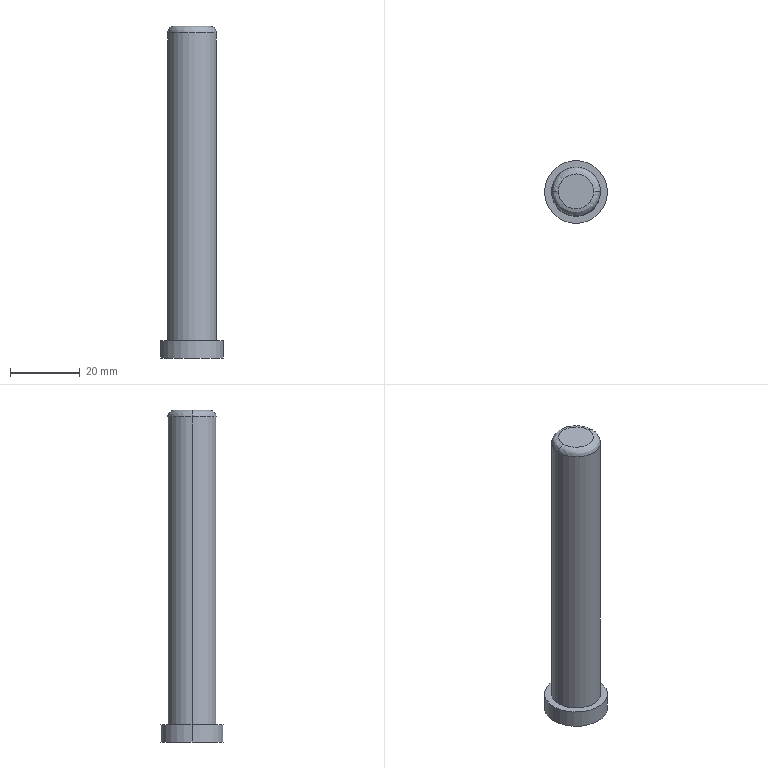Part | STEP file | CHOT DAN DUONG | 1 solid | 9 faces | box 18 x 18 x 95 mm | volume 15092 mm3 | cylinder 4 | plane 3 | spline 2 | commonest cylinder face diameters 14 x2 18 x2
STEP:
#1=CARTESIAN_POINT('',(0.,0.,0.));
#2=DIRECTION('',(0.,0.,1.));
#3=DIRECTION('',(1.,0.,0.));
#4=AXIS2_PLACEMENT_3D('',#1,#2,#3);
#5=CARTESIAN_POINT('',(7.,0.,93.));
#6=VERTEX_POINT('',#5);
#7=CARTESIAN_POINT('',(-7.,0.,93.));
#8=VERTEX_POINT('',#7);
#9=CARTESIAN_POINT('',(0.,0.,93.));
#10=DIRECTION('',(0.,0.,-1.));
#11=DIRECTION('',(1.,0.,0.));
#12=AXIS2_PLACEMENT_3D('',#9,#10,#11);
#13=CIRCLE('',#12,7.);
#14=CARTESIAN_POINT('',(7.,0.,93.));
#15=CARTESIAN_POINT('',(7.,-14.,93.));
#16=CARTESIAN_POINT('',(-7.,-14.,93.));
#17=CARTESIAN_POINT('',(-7.,0.,93.));
#18=CARTESIAN_POINT('',(7.,0.,94.172));
#19=CARTESIAN_POINT('',(7.,-14.,94.172));
#20=CARTESIAN_POINT('',(-7.,-14.,94.172));
#21=CARTESIAN_POINT('',(-7.,0.,94.172));
#22=CARTESIAN_POINT('',(6.172,0.,95.));
#23=CARTESIAN_POINT('',(6.172,-12.343,95.));
#24=CARTESIAN_POINT('',(-6.172,-12.343,95.));
#25=CARTESIAN_POINT('',(-6.172,0.,95.));
#26=CARTESIAN_POINT('',(5.,0.,95.));
#27=CARTESIAN_POINT('',(5.,-10.,95.));
#28=CARTESIAN_POINT('',(-5.,-10.,95.));
#29=CARTESIAN_POINT('',(-5.,0.,95.));
#30=(BOUNDED_SURFACE()B_SPLINE_SURFACE(3,3,((#14,#15,#16,#17),(#18,#19,#20,#21),(#22,#23,#24,#25),(#26,#27,#28,#29)),.UNSPECIFIED.,.F.,.F.,.F.)B_SPLINE_SURFACE_WITH_KNOTS((4,4),(4,4),(0.,1.),(0.,1.),.PIECEWISE_BEZIER_KNOTS.)GEOMETRIC_REPRESENTATION_ITEM()RATIONAL_B_SPLINE_SURFACE(((1.,0.3333,0.3333,1.),(0.8047,0.2682,0.2682,0.8047),(0.8047,0.2682,0.2682,0.8047),(1.,0.3333,0.3333,1.)))REPRESENTATION_ITEM('')SURFACE());
#31=CARTESIAN_POINT('',(0.,0.));
#32=CARTESIAN_POINT('',(0.,0.02375));
#33=CARTESIAN_POINT('',(0.,0.06805));
#34=CARTESIAN_POINT('',(0.,0.1267));
#35=CARTESIAN_POINT('',(0.,0.1794));
#36=CARTESIAN_POINT('',(0.,0.2276));
#37=CARTESIAN_POINT('',(0.,0.2721));
#38=CARTESIAN_POINT('',(0.,0.3139));
#39=CARTESIAN_POINT('',(0.,0.3535));
#40=CARTESIAN_POINT('',(0.,0.3914));
#41=CARTESIAN_POINT('',(0.,0.4282));
#42=CARTESIAN_POINT('',(0.,0.4643));
#43=CARTESIAN_POINT('',(0.,0.5));
#44=CARTESIAN_POINT('',(0.,0.5357));
#45=CARTESIAN_POINT('',(0.,0.5718));
#46=CARTESIAN_POINT('',(0.,0.6086));
#47=CARTESIAN_POINT('',(0.,0.6465));
#48=CARTESIAN_POINT('',(0.,0.6861));
#49=CARTESIAN_POINT('',(0.,0.7279));
#50=CARTESIAN_POINT('',(0.,0.7724));
#51=CARTESIAN_POINT('',(0.,0.8206));
#52=CARTESIAN_POINT('',(0.,0.8733));
#53=CARTESIAN_POINT('',(0.,0.9319));
#54=CARTESIAN_POINT('',(0.,0.9763));
#55=CARTESIAN_POINT('',(0.,1.));
#56=B_SPLINE_CURVE_WITH_KNOTS('',3,(#31,#32,#33,#34,#35,#36,#37,#38,#39,#40,#41,#42,#43,#44,#45,#46,#47,#48,#49,#50,#51,#52,#53,#54,#55),.UNSPECIFIED.,.F.,.F.,(4,1,1,1,1,1,1,1,1,1,1,1,1,1,1,1,1,1,1,1,1,1,4),(0.,0.1428,0.2856,0.4284,0.5712,0.714,0.8568,0.9996,1.142,1.285,1.428,1.571,1.714,1.856,1.999,2.142,2.285,2.428,2.57,2.713,2.856,2.999,3.142),.QUASI_UNIFORM_KNOTS.);
#57=(GEOMETRIC_REPRESENTATION_CONTEXT(2)PARAMETRIC_REPRESENTATION_CONTEXT()REPRESENTATION_CONTEXT('',''));
#58=DEFINITIONAL_REPRESENTATION('',(#56),#57);
#59=PCURVE('',#30,#58);
#60=CARTESIAN_POINT('',(0.,0.,5.));
#61=DIRECTION('',(0.,0.,1.));
#62=DIRECTION('',(1.,0.,0.));
#63=AXIS2_PLACEMENT_3D('',#60,#61,#62);
#64=CYLINDRICAL_SURFACE('',#63,7.);
#65=CARTESIAN_POINT('',(6.283,88.));
#66=DIRECTION('',(-1.,0.));
#67=VECTOR('',#66,1.);
#68=LINE('',#65,#67);
#69=(GEOMETRIC_REPRESENTATION_CONTEXT(2)PARAMETRIC_REPRESENTATION_CONTEXT()REPRESENTATION_CONTEXT('',''));
#70=DEFINITIONAL_REPRESENTATION('',(#68),#69);
#71=PCURVE('',#64,#70);
#72=SURFACE_CURVE('',#13,(#59,#71),.PCURVE_S1.);
#73=EDGE_CURVE('',#6,#8,#72,.T.);
#74=ORIENTED_EDGE('',*,*,#73,.F.);
#75=CARTESIAN_POINT('',(5.,0.,95.));
#76=VERTEX_POINT('',#75);
#77=CARTESIAN_POINT('',(5.,0.,93.));
#78=DIRECTION('',(0.,-1.,0.));
#79=DIRECTION('',(1.,0.,0.));
#80=AXIS2_PLACEMENT_3D('',#77,#78,#79);
#81=CIRCLE('',#80,2.);
#82=CARTESIAN_POINT('',(0.,0.));
#83=CARTESIAN_POINT('',(0.01683,0.));
#84=CARTESIAN_POINT('',(0.04999,0.));
#85=CARTESIAN_POINT('',(0.09843,0.));
#86=CARTESIAN_POINT('',(0.1457,0.));
#87=CARTESIAN_POINT('',(0.192,0.));
#88=CARTESIAN_POINT('',(0.2375,0.));
#89=CARTESIAN_POINT('',(0.2823,0.));
#90=CARTESIAN_POINT('',(0.3265,0.));
#91=CARTESIAN_POINT('',(0.3703,0.));
#92=CARTESIAN_POINT('',(0.4137,0.));
#93=CARTESIAN_POINT('',(0.4569,0.));
#94=CARTESIAN_POINT('',(0.5,0.));
#95=CARTESIAN_POINT('',(0.5431,0.));
#96=CARTESIAN_POINT('',(0.5863,0.));
#97=CARTESIAN_POINT('',(0.6297,0.));
#98=CARTESIAN_POINT('',(0.6735,0.));
#99=CARTESIAN_POINT('',(0.7177,0.));
#100=CARTESIAN_POINT('',(0.7625,0.));
#101=CARTESIAN_POINT('',(0.808,0.));
#102=CARTESIAN_POINT('',(0.8543,0.));
#103=CARTESIAN_POINT('',(0.9016,0.));
#104=CARTESIAN_POINT('',(0.95,0.));
#105=CARTESIAN_POINT('',(0.9832,0.));
#106=CARTESIAN_POINT('',(1.,0.));
#107=B_SPLINE_CURVE_WITH_KNOTS('',3,(#82,#83,#84,#85,#86,#87,#88,#89,#90,#91,#92,#93,#94,#95,#96,#97,#98,#99,#100,#101,#102,#103,#104,#105,#106),.UNSPECIFIED.,.F.,.F.,(4,1,1,1,1,1,1,1,1,1,1,1,1,1,1,1,1,1,1,1,1,1,4),(0.,0.0714,0.1428,0.2142,0.2856,0.357,0.4284,0.4998,0.5712,0.6426,0.714,0.7854,0.8568,0.9282,0.9996,1.071,1.142,1.214,1.285,1.357,1.428,1.499,1.571),.QUASI_UNIFORM_KNOTS.);
#108=(GEOMETRIC_REPRESENTATION_CONTEXT(2)PARAMETRIC_REPRESENTATION_CONTEXT()REPRESENTATION_CONTEXT('',''));
#109=DEFINITIONAL_REPRESENTATION('',(#107),#108);
#110=PCURVE('',#30,#109);
#111=CARTESIAN_POINT('',(-7.,0.,93.));
#112=CARTESIAN_POINT('',(-7.,14.,93.));
#113=CARTESIAN_POINT('',(7.,14.,93.));
#114=CARTESIAN_POINT('',(7.,0.,93.));
#115=CARTESIAN_POINT('',(-7.,0.,94.172));
#116=CARTESIAN_POINT('',(-7.,14.,94.172));
#117=CARTESIAN_POINT('',(7.,14.,94.172));
#118=CARTESIAN_POINT('',(7.,0.,94.172));
#119=CARTESIAN_POINT('',(-6.172,0.,95.));
#120=CARTESIAN_POINT('',(-6.172,12.343,95.));
#121=CARTESIAN_POINT('',(6.172,12.343,95.));
#122=CARTESIAN_POINT('',(6.172,0.,95.));
#123=CARTESIAN_POINT('',(-5.,0.,95.));
#124=CARTESIAN_POINT('',(-5.,10.,95.));
#125=CARTESIAN_POINT('',(5.,10.,95.));
#126=CARTESIAN_POINT('',(5.,0.,95.));
#127=(BOUNDED_SURFACE()B_SPLINE_SURFACE(3,3,((#111,#112,#113,#114),(#115,#116,#117,#118),(#119,#120,#121,#122),(#123,#124,#125,#126)),.UNSPECIFIED.,.F.,.F.,.F.)B_SPLINE_SURFACE_WITH_KNOTS((4,4),(4,4),(0.,1.),(0.,1.),.PIECEWISE_BEZIER_KNOTS.)GEOMETRIC_REPRESENTATION_ITEM()RATIONAL_B_SPLINE_SURFACE(((1.,0.3333,0.3333,1.),(0.8047,0.2682,0.2682,0.8047),(0.8047,0.2682,0.2682,0.8047),(1.,0.3333,0.3333,1.)))REPRESENTATION_ITEM('')SURFACE());
#128=CARTESIAN_POINT('',(0.,1.));
#129=CARTESIAN_POINT('',(0.01683,1.));
#130=CARTESIAN_POINT('',(0.04999,1.));
#131=CARTESIAN_POINT('',(0.09843,1.));
#132=CARTESIAN_POINT('',(0.1457,1.));
#133=CARTESIAN_POINT('',(0.192,1.));
#134=CARTESIAN_POINT('',(0.2375,1.));
#135=CARTESIAN_POINT('',(0.2823,1.));
#136=CARTESIAN_POINT('',(0.3265,1.));
#137=CARTESIAN_POINT('',(0.3703,1.));
#138=CARTESIAN_POINT('',(0.4137,1.));
#139=CARTESIAN_POINT('',(0.4569,1.));
#140=CARTESIAN_POINT('',(0.5,1.));
#141=CARTESIAN_POINT('',(0.5431,1.));
#142=CARTESIAN_POINT('',(0.5863,1.));
#143=CARTESIAN_POINT('',(0.6297,1.));
#144=CARTESIAN_POINT('',(0.6735,1.));
#145=CARTESIAN_POINT('',(0.7177,1.));
#146=CARTESIAN_POINT('',(0.7625,1.));
#147=CARTESIAN_POINT('',(0.808,1.));
#148=CARTESIAN_POINT('',(0.8543,1.));
#149=CARTESIAN_POINT('',(0.9016,1.));
#150=CARTESIAN_POINT('',(0.95,1.));
#151=CARTESIAN_POINT('',(0.9832,1.));
#152=CARTESIAN_POINT('',(1.,1.));
#153=B_SPLINE_CURVE_WITH_KNOTS('',3,(#128,#129,#130,#131,#132,#133,#134,#135,#136,#137,#138,#139,#140,#141,#142,#143,#144,#145,#146,#147,#148,#149,#150,#151,#152),.UNSPECIFIED.,.F.,.F.,(4,1,1,1,1,1,1,1,1,1,1,1,1,1,1,1,1,1,1,1,1,1,4),(0.,0.0714,0.1428,0.2142,0.2856,0.357,0.4284,0.4998,0.5712,0.6426,0.714,0.7854,0.8568,0.9282,0.9996,1.071,1.142,1.214,1.285,1.357,1.428,1.499,1.571),.QUASI_UNIFORM_KNOTS.);
#154=(GEOMETRIC_REPRESENTATION_CONTEXT(2)PARAMETRIC_REPRESENTATION_CONTEXT()REPRESENTATION_CONTEXT('',''));
#155=DEFINITIONAL_REPRESENTATION('',(#153),#154);
#156=PCURVE('',#127,#155);
#157=SURFACE_CURVE('',#81,(#110,#156),.PCURVE_S1.);
#158=EDGE_CURVE('',#6,#76,#157,.T.);
#159=ORIENTED_EDGE('',*,*,#158,.T.);
#160=CARTESIAN_POINT('',(-5.,0.,95.));
#161=VERTEX_POINT('',#160);
#162=CARTESIAN_POINT('',(5.,0.,95.));
#163=CARTESIAN_POINT('',(5.,-10.,95.));
#164=CARTESIAN_POINT('',(-5.,-10.,95.));
#165=CARTESIAN_POINT('',(-5.,0.,95.));
#166=(BOUNDED_CURVE()B_SPLINE_CURVE(3,(#162,#163,#164,#165),.UNSPECIFIED.,.F.,.F.)B_SPLINE_CURVE_WITH_KNOTS((4,4),(0.,0.5),.PIECEWISE_BEZIER_KNOTS.)CURVE()GEOMETRIC_REPRESENTATION_ITEM()RATIONAL_B_SPLINE_CURVE((1.,0.3333,0.3333,1.))REPRESENTATION_ITEM(''));
#167=CARTESIAN_POINT('',(1.,0.));
#168=CARTESIAN_POINT('',(1.,1.));
#169=B_SPLINE_CURVE_WITH_KNOTS('',1,(#167,#168),.UNSPECIFIED.,.F.,.F.,(2,2),(0.,0.5),.PIECEWISE_BEZIER_KNOTS.);
#170=(GEOMETRIC_REPRESENTATION_CONTEXT(2)PARAMETRIC_REPRESENTATION_CONTEXT()REPRESENTATION_CONTEXT('',''));
#171=DEFINITIONAL_REPRESENTATION('',(#169),#170);
#172=PCURVE('',#30,#171);
#173=CARTESIAN_POINT('',(0.,0.,95.));
#174=DIRECTION('',(0.,0.,-1.));
#175=DIRECTION('',(-1.,0.,0.));
#176=AXIS2_PLACEMENT_3D('',#173,#174,#175);
#177=PLANE('',#176);
#178=CARTESIAN_POINT('',(-5.,0.));
#179=CARTESIAN_POINT('',(-5.,-10.));
#180=CARTESIAN_POINT('',(5.,-10.));
#181=CARTESIAN_POINT('',(5.,0.));
#182=(BOUNDED_CURVE()B_SPLINE_CURVE(3,(#178,#179,#180,#181),.UNSPECIFIED.,.F.,.F.)B_SPLINE_CURVE_WITH_KNOTS((4,4),(0.,0.5),.PIECEWISE_BEZIER_KNOTS.)CURVE()GEOMETRIC_REPRESENTATION_ITEM()RATIONAL_B_SPLINE_CURVE((1.,0.3333,0.3333,1.))REPRESENTATION_ITEM(''));
#183=(GEOMETRIC_REPRESENTATION_CONTEXT(2)PARAMETRIC_REPRESENTATION_CONTEXT()REPRESENTATION_CONTEXT('',''));
#184=DEFINITIONAL_REPRESENTATION('',(#182),#183);
#185=PCURVE('',#177,#184);
#186=SURFACE_CURVE('',#166,(#172,#185),.PCURVE_S1.);
#187=EDGE_CURVE('',#76,#161,#186,.T.);
#188=ORIENTED_EDGE('',*,*,#187,.T.);
#189=CARTESIAN_POINT('',(-5.,0.,93.));
#190=DIRECTION('',(0.,1.,0.));
#191=DIRECTION('',(-1.,0.,0.));
#192=AXIS2_PLACEMENT_3D('',#189,#190,#191);
#193=CIRCLE('',#192,2.);
#194=CARTESIAN_POINT('',(0.,1.));
#195=CARTESIAN_POINT('',(0.01683,1.));
#196=CARTESIAN_POINT('',(0.04999,1.));
#197=CARTESIAN_POINT('',(0.09843,1.));
#198=CARTESIAN_POINT('',(0.1457,1.));
#199=CARTESIAN_POINT('',(0.192,1.));
#200=CARTESIAN_POINT('',(0.2375,1.));
#201=CARTESIAN_POINT('',(0.2823,1.));
#202=CARTESIAN_POINT('',(0.3265,1.));
#203=CARTESIAN_POINT('',(0.3703,1.));
#204=CARTESIAN_POINT('',(0.4137,1.));
#205=CARTESIAN_POINT('',(0.4569,1.));
#206=CARTESIAN_POINT('',(0.5,1.));
#207=CARTESIAN_POINT('',(0.5431,1.));
#208=CARTESIAN_POINT('',(0.5863,1.));
#209=CARTESIAN_POINT('',(0.6297,1.));
#210=CARTESIAN_POINT('',(0.6735,1.));
#211=CARTESIAN_POINT('',(0.7177,1.));
#212=CARTESIAN_POINT('',(0.7625,1.));
#213=CARTESIAN_POINT('',(0.808,1.));
#214=CARTESIAN_POINT('',(0.8543,1.));
#215=CARTESIAN_POINT('',(0.9016,1.));
#216=CARTESIAN_POINT('',(0.95,1.));
#217=CARTESIAN_POINT('',(0.9832,1.));
#218=CARTESIAN_POINT('',(1.,1.));
#219=B_SPLINE_CURVE_WITH_KNOTS('',3,(#194,#195,#196,#197,#198,#199,#200,#201,#202,#203,#204,#205,#206,#207,#208,#209,#210,#211,#212,#213,#214,#215,#216,#217,#218),.UNSPECIFIED.,.F.,.F.,(4,1,1,1,1,1,1,1,1,1,1,1,1,1,1,1,1,1,1,1,1,1,4),(0.,0.0714,0.1428,0.2142,0.2856,0.357,0.4284,0.4998,0.5712,0.6426,0.714,0.7854,0.8568,0.9282,0.9996,1.071,1.142,1.214,1.285,1.357,1.428,1.499,1.571),.QUASI_UNIFORM_KNOTS.);
#220=(GEOMETRIC_REPRESENTATION_CONTEXT(2)PARAMETRIC_REPRESENTATION_CONTEXT()REPRESENTATION_CONTEXT('',''));
#221=DEFINITIONAL_REPRESENTATION('',(#219),#220);
#222=PCURVE('',#30,#221);
#223=CARTESIAN_POINT('',(0.,0.));
#224=CARTESIAN_POINT('',(0.01683,0.));
#225=CARTESIAN_POINT('',(0.04999,0.));
#226=CARTESIAN_POINT('',(0.09843,0.));
#227=CARTESIAN_POINT('',(0.1457,0.));
#228=CARTESIAN_POINT('',(0.192,0.));
#229=CARTESIAN_POINT('',(0.2375,0.));
#230=CARTESIAN_POINT('',(0.2823,0.));
#231=CARTESIAN_POINT('',(0.3265,0.));
#232=CARTESIAN_POINT('',(0.3703,0.));
#233=CARTESIAN_POINT('',(0.4137,0.));
#234=CARTESIAN_POINT('',(0.4569,0.));
#235=CARTESIAN_POINT('',(0.5,0.));
#236=CARTESIAN_POINT('',(0.5431,0.));
#237=CARTESIAN_POINT('',(0.5863,0.));
#238=CARTESIAN_POINT('',(0.6297,0.));
#239=CARTESIAN_POINT('',(0.6735,0.));
#240=CARTESIAN_POINT('',(0.7177,0.));
#241=CARTESIAN_POINT('',(0.7625,0.));
#242=CARTESIAN_POINT('',(0.808,0.));
#243=CARTESIAN_POINT('',(0.8543,0.));
#244=CARTESIAN_POINT('',(0.9016,0.));
#245=CARTESIAN_POINT('',(0.95,0.));
#246=CARTESIAN_POINT('',(0.9832,0.));
#247=CARTESIAN_POINT('',(1.,0.));
#248=B_SPLINE_CURVE_WITH_KNOTS('',3,(#223,#224,#225,#226,#227,#228,#229,#230,#231,#232,#233,#234,#235,#236,#237,#238,#239,#240,#241,#242,#243,#244,#245,#246,#247),.UNSPECIFIED.,.F.,.F.,(4,1,1,1,1,1,1,1,1,1,1,1,1,1,1,1,1,1,1,1,1,1,4),(0.,0.0714,0.1428,0.2142,0.2856,0.357,0.4284,0.4998,0.5712,0.6426,0.714,0.7854,0.8568,0.9282,0.9996,1.071,1.142,1.214,1.285,1.357,1.428,1.499,1.571),.QUASI_UNIFORM_KNOTS.);
#249=(GEOMETRIC_REPRESENTATION_CONTEXT(2)PARAMETRIC_REPRESENTATION_CONTEXT()REPRESENTATION_CONTEXT('',''));
#250=DEFINITIONAL_REPRESENTATION('',(#248),#249);
#251=PCURVE('',#127,#250);
#252=SURFACE_CURVE('',#193,(#222,#251),.PCURVE_S1.);
#253=EDGE_CURVE('',#8,#161,#252,.T.);
#254=ORIENTED_EDGE('',*,*,#253,.F.);
#255=EDGE_LOOP('',(#74,#159,#188,#254));
#256=FACE_BOUND('',#255,.T.);
#257=ADVANCED_FACE('',(#256),#30,.T.);
#258=CARTESIAN_POINT('',(7.,0.,5.));
#259=VERTEX_POINT('',#258);
#260=CARTESIAN_POINT('',(-7.,0.,5.));
#261=VERTEX_POINT('',#260);
#262=CARTESIAN_POINT('',(0.,0.,5.));
#263=DIRECTION('',(0.,0.,1.));
#264=DIRECTION('',(1.,0.,0.));
#265=AXIS2_PLACEMENT_3D('',#262,#263,#264);
#266=CIRCLE('',#265,7.);
#267=CARTESIAN_POINT('',(0.,0.,5.));
#268=DIRECTION('',(0.,0.,1.));
#269=DIRECTION('',(1.,0.,0.));
#270=AXIS2_PLACEMENT_3D('',#267,#268,#269);
#271=CYLINDRICAL_SURFACE('',#270,7.);
#272=CARTESIAN_POINT('',(0.,0.));
#273=DIRECTION('',(1.,0.));
#274=VECTOR('',#273,1.);
#275=LINE('',#272,#274);
#276=(GEOMETRIC_REPRESENTATION_CONTEXT(2)PARAMETRIC_REPRESENTATION_CONTEXT()REPRESENTATION_CONTEXT('',''));
#277=DEFINITIONAL_REPRESENTATION('',(#275),#276);
#278=PCURVE('',#271,#277);
#279=CARTESIAN_POINT('',(0.,0.,5.));
#280=DIRECTION('',(0.,0.,-1.));
#281=DIRECTION('',(-1.,0.,0.));
#282=AXIS2_PLACEMENT_3D('',#279,#280,#281);
#283=PLANE('',#282);
#284=CARTESIAN_POINT('',(-7.,0.));
#285=CARTESIAN_POINT('',(-7.,12.124));
#286=CARTESIAN_POINT('',(3.5,6.062));
#287=CARTESIAN_POINT('',(14.,0.));
#288=CARTESIAN_POINT('',(3.5,-6.062));
#289=CARTESIAN_POINT('',(-7.,-12.124));
#290=CARTESIAN_POINT('',(-7.,0.));
#291=(BOUNDED_CURVE()B_SPLINE_CURVE(2,(#284,#285,#286,#287,#288,#289,#290),.UNSPECIFIED.,.T.,.F.)B_SPLINE_CURVE_WITH_KNOTS((1,2,2,2,2,1),(-2.094,0.,2.094,4.189,6.283,8.378),.UNSPECIFIED.)CURVE()GEOMETRIC_REPRESENTATION_ITEM()RATIONAL_B_SPLINE_CURVE((1.,0.5,1.,0.5,1.,0.5,1.))REPRESENTATION_ITEM(''));
#292=(GEOMETRIC_REPRESENTATION_CONTEXT(2)PARAMETRIC_REPRESENTATION_CONTEXT()REPRESENTATION_CONTEXT('',''));
#293=DEFINITIONAL_REPRESENTATION('',(#291),#292);
#294=PCURVE('',#283,#293);
#295=SURFACE_CURVE('',#266,(#278,#294),.PCURVE_S1.);
#296=EDGE_CURVE('',#259,#261,#295,.T.);
#297=ORIENTED_EDGE('',*,*,#296,.T.);
#298=CARTESIAN_POINT('',(-7.,0.,5.));
#299=DIRECTION('',(0.,0.,1.));
#300=VECTOR('',#299,1.);
#301=LINE('',#298,#300);
#302=CARTESIAN_POINT('',(3.142,0.));
#303=DIRECTION('',(0.,1.));
#304=VECTOR('',#303,1.);
#305=LINE('',#302,#304);
#306=(GEOMETRIC_REPRESENTATION_CONTEXT(2)PARAMETRIC_REPRESENTATION_CONTEXT()REPRESENTATION_CONTEXT('',''));
#307=DEFINITIONAL_REPRESENTATION('',(#305),#306);
#308=PCURVE('',#271,#307);
#309=CARTESIAN_POINT('',(3.142,0.));
#310=DIRECTION('',(0.,1.));
#311=VECTOR('',#310,1.);
#312=LINE('',#309,#311);
#313=(GEOMETRIC_REPRESENTATION_CONTEXT(2)PARAMETRIC_REPRESENTATION_CONTEXT()REPRESENTATION_CONTEXT('',''));
#314=DEFINITIONAL_REPRESENTATION('',(#312),#313);
#315=PCURVE('',#64,#314);
#316=SURFACE_CURVE('',#301,(#308,#315),.PCURVE_S1.);
#317=EDGE_CURVE('',#261,#8,#316,.T.);
#318=ORIENTED_EDGE('',*,*,#317,.T.);
#319=CARTESIAN_POINT('',(0.,0.,93.));
#320=DIRECTION('',(0.,0.,-1.));
#321=DIRECTION('',(1.,0.,0.));
#322=AXIS2_PLACEMENT_3D('',#319,#320,#321);
#323=CIRCLE('',#322,7.);
#324=CARTESIAN_POINT('',(6.283,88.));
#325=DIRECTION('',(-1.,0.));
#326=VECTOR('',#325,1.);
#327=LINE('',#324,#326);
#328=(GEOMETRIC_REPRESENTATION_CONTEXT(2)PARAMETRIC_REPRESENTATION_CONTEXT()REPRESENTATION_CONTEXT('',''));
#329=DEFINITIONAL_REPRESENTATION('',(#327),#328);
#330=PCURVE('',#271,#329);
#331=CARTESIAN_POINT('',(0.,0.));
#332=CARTESIAN_POINT('',(0.,0.02375));
#333=CARTESIAN_POINT('',(0.,0.06805));
#334=CARTESIAN_POINT('',(0.,0.1267));
#335=CARTESIAN_POINT('',(0.,0.1794));
#336=CARTESIAN_POINT('',(0.,0.2276));
#337=CARTESIAN_POINT('',(0.,0.2721));
#338=CARTESIAN_POINT('',(0.,0.3139));
#339=CARTESIAN_POINT('',(0.,0.3535));
#340=CARTESIAN_POINT('',(0.,0.3914));
#341=CARTESIAN_POINT('',(0.,0.4282));
#342=CARTESIAN_POINT('',(0.,0.4643));
#343=CARTESIAN_POINT('',(0.,0.5));
#344=CARTESIAN_POINT('',(0.,0.5357));
#345=CARTESIAN_POINT('',(0.,0.5718));
#346=CARTESIAN_POINT('',(0.,0.6086));
#347=CARTESIAN_POINT('',(0.,0.6465));
#348=CARTESIAN_POINT('',(0.,0.6861));
#349=CARTESIAN_POINT('',(0.,0.7279));
#350=CARTESIAN_POINT('',(0.,0.7724));
#351=CARTESIAN_POINT('',(0.,0.8206));
#352=CARTESIAN_POINT('',(0.,0.8733));
#353=CARTESIAN_POINT('',(0.,0.9319));
#354=CARTESIAN_POINT('',(0.,0.9763));
#355=CARTESIAN_POINT('',(0.,1.));
#356=B_SPLINE_CURVE_WITH_KNOTS('',3,(#331,#332,#333,#334,#335,#336,#337,#338,#339,#340,#341,#342,#343,#344,#345,#346,#347,#348,#349,#350,#351,#352,#353,#354,#355),.UNSPECIFIED.,.F.,.F.,(4,1,1,1,1,1,1,1,1,1,1,1,1,1,1,1,1,1,1,1,1,1,4),(3.142,3.284,3.427,3.57,3.713,3.856,3.998,4.141,4.284,4.427,4.57,4.712,4.855,4.998,5.141,5.284,5.426,5.569,5.712,5.855,5.998,6.14,6.283),.QUASI_UNIFORM_KNOTS.);
#357=(GEOMETRIC_REPRESENTATION_CONTEXT(2)PARAMETRIC_REPRESENTATION_CONTEXT()REPRESENTATION_CONTEXT('',''));
#358=DEFINITIONAL_REPRESENTATION('',(#356),#357);
#359=PCURVE('',#127,#358);
#360=SURFACE_CURVE('',#323,(#330,#359),.PCURVE_S1.);
#361=EDGE_CURVE('',#8,#6,#360,.T.);
#362=ORIENTED_EDGE('',*,*,#361,.T.);
#363=CARTESIAN_POINT('',(7.,0.,5.));
#364=DIRECTION('',(0.,0.,1.));
#365=VECTOR('',#364,1.);
#366=LINE('',#363,#365);
#367=CARTESIAN_POINT('',(0.,0.));
#368=DIRECTION('',(0.,1.));
#369=VECTOR('',#368,1.);
#370=LINE('',#367,#369);
#371=(GEOMETRIC_REPRESENTATION_CONTEXT(2)PARAMETRIC_REPRESENTATION_CONTEXT()REPRESENTATION_CONTEXT('',''));
#372=DEFINITIONAL_REPRESENTATION('',(#370),#371);
#373=PCURVE('',#271,#372);
#374=CARTESIAN_POINT('',(6.283,0.));
#375=DIRECTION('',(0.,1.));
#376=VECTOR('',#375,1.);
#377=LINE('',#374,#376);
#378=(GEOMETRIC_REPRESENTATION_CONTEXT(2)PARAMETRIC_REPRESENTATION_CONTEXT()REPRESENTATION_CONTEXT('',''));
#379=DEFINITIONAL_REPRESENTATION('',(#377),#378);
#380=PCURVE('',#64,#379);
#381=SURFACE_CURVE('',#366,(#373,#380),.PCURVE_S1.);
#382=EDGE_CURVE('',#259,#6,#381,.T.);
#383=ORIENTED_EDGE('',*,*,#382,.F.);
#384=EDGE_LOOP('',(#297,#318,#362,#383));
#385=FACE_BOUND('',#384,.T.);
#386=ADVANCED_FACE('',(#385),#271,.T.);
#387=CARTESIAN_POINT('',(9.,0.,0.));
#388=VERTEX_POINT('',#387);
#389=CARTESIAN_POINT('',(-9.,0.,0.));
#390=VERTEX_POINT('',#389);
#391=CARTESIAN_POINT('',(0.,0.,0.));
#392=DIRECTION('',(0.,0.,1.));
#393=DIRECTION('',(1.,0.,0.));
#394=AXIS2_PLACEMENT_3D('',#391,#392,#393);
#395=CIRCLE('',#394,9.);
#396=CARTESIAN_POINT('',(0.,0.,0.));
#397=DIRECTION('',(0.,0.,1.));
#398=DIRECTION('',(1.,0.,0.));
#399=AXIS2_PLACEMENT_3D('',#396,#397,#398);
#400=CYLINDRICAL_SURFACE('',#399,9.);
#401=CARTESIAN_POINT('',(0.,0.));
#402=DIRECTION('',(1.,0.));
#403=VECTOR('',#402,1.);
#404=LINE('',#401,#403);
#405=(GEOMETRIC_REPRESENTATION_CONTEXT(2)PARAMETRIC_REPRESENTATION_CONTEXT()REPRESENTATION_CONTEXT('',''));
#406=DEFINITIONAL_REPRESENTATION('',(#404),#405);
#407=PCURVE('',#400,#406);
#408=CARTESIAN_POINT('',(0.,0.,0.));
#409=DIRECTION('',(0.,0.,-1.));
#410=DIRECTION('',(-1.,0.,0.));
#411=AXIS2_PLACEMENT_3D('',#408,#409,#410);
#412=PLANE('',#411);
#413=CARTESIAN_POINT('',(-9.,0.));
#414=CARTESIAN_POINT('',(-9.,15.588));
#415=CARTESIAN_POINT('',(4.5,7.794));
#416=CARTESIAN_POINT('',(18.,0.));
#417=CARTESIAN_POINT('',(4.5,-7.794));
#418=CARTESIAN_POINT('',(-9.,-15.588));
#419=CARTESIAN_POINT('',(-9.,0.));
#420=(BOUNDED_CURVE()B_SPLINE_CURVE(2,(#413,#414,#415,#416,#417,#418,#419),.UNSPECIFIED.,.T.,.F.)B_SPLINE_CURVE_WITH_KNOTS((1,2,2,2,2,1),(-2.094,0.,2.094,4.189,6.283,8.378),.UNSPECIFIED.)CURVE()GEOMETRIC_REPRESENTATION_ITEM()RATIONAL_B_SPLINE_CURVE((1.,0.5,1.,0.5,1.,0.5,1.))REPRESENTATION_ITEM(''));
#421=(GEOMETRIC_REPRESENTATION_CONTEXT(2)PARAMETRIC_REPRESENTATION_CONTEXT()REPRESENTATION_CONTEXT('',''));
#422=DEFINITIONAL_REPRESENTATION('',(#420),#421);
#423=PCURVE('',#412,#422);
#424=SURFACE_CURVE('',#395,(#407,#423),.PCURVE_S1.);
#425=EDGE_CURVE('',#388,#390,#424,.T.);
#426=ORIENTED_EDGE('',*,*,#425,.T.);
#427=CARTESIAN_POINT('',(-9.,0.,5.));
#428=VERTEX_POINT('',#427);
#429=CARTESIAN_POINT('',(-9.,0.,0.));
#430=DIRECTION('',(0.,0.,1.));
#431=VECTOR('',#430,1.);
#432=LINE('',#429,#431);
#433=CARTESIAN_POINT('',(3.142,0.));
#434=DIRECTION('',(0.,1.));
#435=VECTOR('',#434,1.);
#436=LINE('',#433,#435);
#437=(GEOMETRIC_REPRESENTATION_CONTEXT(2)PARAMETRIC_REPRESENTATION_CONTEXT()REPRESENTATION_CONTEXT('',''));
#438=DEFINITIONAL_REPRESENTATION('',(#436),#437);
#439=PCURVE('',#400,#438);
#440=CARTESIAN_POINT('',(0.,0.,0.));
#441=DIRECTION('',(0.,0.,1.));
#442=DIRECTION('',(1.,0.,0.));
#443=AXIS2_PLACEMENT_3D('',#440,#441,#442);
#444=CYLINDRICAL_SURFACE('',#443,9.);
#445=CARTESIAN_POINT('',(3.142,0.));
#446=DIRECTION('',(0.,1.));
#447=VECTOR('',#446,1.);
#448=LINE('',#445,#447);
#449=(GEOMETRIC_REPRESENTATION_CONTEXT(2)PARAMETRIC_REPRESENTATION_CONTEXT()REPRESENTATION_CONTEXT('',''));
#450=DEFINITIONAL_REPRESENTATION('',(#448),#449);
#451=PCURVE('',#444,#450);
#452=SURFACE_CURVE('',#432,(#439,#451),.PCURVE_S1.);
#453=EDGE_CURVE('',#390,#428,#452,.T.);
#454=ORIENTED_EDGE('',*,*,#453,.T.);
#455=CARTESIAN_POINT('',(9.,0.,5.));
#456=VERTEX_POINT('',#455);
#457=CARTESIAN_POINT('',(0.,0.,5.));
#458=DIRECTION('',(0.,0.,-1.));
#459=DIRECTION('',(1.,0.,0.));
#460=AXIS2_PLACEMENT_3D('',#457,#458,#459);
#461=CIRCLE('',#460,9.);
#462=CARTESIAN_POINT('',(6.283,5.));
#463=DIRECTION('',(-1.,0.));
#464=VECTOR('',#463,1.);
#465=LINE('',#462,#464);
#466=(GEOMETRIC_REPRESENTATION_CONTEXT(2)PARAMETRIC_REPRESENTATION_CONTEXT()REPRESENTATION_CONTEXT('',''));
#467=DEFINITIONAL_REPRESENTATION('',(#465),#466);
#468=PCURVE('',#400,#467);
#469=CARTESIAN_POINT('',(0.,0.));
#470=DIRECTION('',(-1.,0.));
#471=AXIS2_PLACEMENT_2D('',#469,#470);
#472=CIRCLE('',#471,9.);
#473=(GEOMETRIC_REPRESENTATION_CONTEXT(2)PARAMETRIC_REPRESENTATION_CONTEXT()REPRESENTATION_CONTEXT('',''));
#474=DEFINITIONAL_REPRESENTATION('',(#472),#473);
#475=PCURVE('',#283,#474);
#476=SURFACE_CURVE('',#461,(#468,#475),.PCURVE_S1.);
#477=EDGE_CURVE('',#428,#456,#476,.T.);
#478=ORIENTED_EDGE('',*,*,#477,.T.);
#479=CARTESIAN_POINT('',(9.,0.,0.));
#480=DIRECTION('',(0.,0.,1.));
#481=VECTOR('',#480,1.);
#482=LINE('',#479,#481);
#483=CARTESIAN_POINT('',(0.,0.));
#484=DIRECTION('',(0.,1.));
#485=VECTOR('',#484,1.);
#486=LINE('',#483,#485);
#487=(GEOMETRIC_REPRESENTATION_CONTEXT(2)PARAMETRIC_REPRESENTATION_CONTEXT()REPRESENTATION_CONTEXT('',''));
#488=DEFINITIONAL_REPRESENTATION('',(#486),#487);
#489=PCURVE('',#400,#488);
#490=CARTESIAN_POINT('',(6.283,0.));
#491=DIRECTION('',(0.,1.));
#492=VECTOR('',#491,1.);
#493=LINE('',#490,#492);
#494=(GEOMETRIC_REPRESENTATION_CONTEXT(2)PARAMETRIC_REPRESENTATION_CONTEXT()REPRESENTATION_CONTEXT('',''));
#495=DEFINITIONAL_REPRESENTATION('',(#493),#494);
#496=PCURVE('',#444,#495);
#497=SURFACE_CURVE('',#482,(#489,#496),.PCURVE_S1.);
#498=EDGE_CURVE('',#388,#456,#497,.T.);
#499=ORIENTED_EDGE('',*,*,#498,.F.);
#500=EDGE_LOOP('',(#426,#454,#478,#499));
#501=FACE_BOUND('',#500,.T.);
#502=ADVANCED_FACE('',(#501),#400,.T.);
#503=ORIENTED_EDGE('',*,*,#317,.F.);
#504=CARTESIAN_POINT('',(0.,0.,5.));
#505=DIRECTION('',(0.,0.,1.));
#506=DIRECTION('',(1.,0.,0.));
#507=AXIS2_PLACEMENT_3D('',#504,#505,#506);
#508=CIRCLE('',#507,7.);
#509=CARTESIAN_POINT('',(0.,0.));
#510=DIRECTION('',(1.,0.));
#511=VECTOR('',#510,1.);
#512=LINE('',#509,#511);
#513=(GEOMETRIC_REPRESENTATION_CONTEXT(2)PARAMETRIC_REPRESENTATION_CONTEXT()REPRESENTATION_CONTEXT('',''));
#514=DEFINITIONAL_REPRESENTATION('',(#512),#513);
#515=PCURVE('',#64,#514);
#516=CARTESIAN_POINT('',(-7.,0.));
#517=CARTESIAN_POINT('',(-7.,12.124));
#518=CARTESIAN_POINT('',(3.5,6.062));
#519=CARTESIAN_POINT('',(14.,0.));
#520=CARTESIAN_POINT('',(3.5,-6.062));
#521=CARTESIAN_POINT('',(-7.,-12.124));
#522=CARTESIAN_POINT('',(-7.,0.));
#523=(BOUNDED_CURVE()B_SPLINE_CURVE(2,(#516,#517,#518,#519,#520,#521,#522),.UNSPECIFIED.,.T.,.F.)B_SPLINE_CURVE_WITH_KNOTS((1,2,2,2,2,1),(-2.094,0.,2.094,4.189,6.283,8.378),.UNSPECIFIED.)CURVE()GEOMETRIC_REPRESENTATION_ITEM()RATIONAL_B_SPLINE_CURVE((1.,0.5,1.,0.5,1.,0.5,1.))REPRESENTATION_ITEM(''));
#524=(GEOMETRIC_REPRESENTATION_CONTEXT(2)PARAMETRIC_REPRESENTATION_CONTEXT()REPRESENTATION_CONTEXT('',''));
#525=DEFINITIONAL_REPRESENTATION('',(#523),#524);
#526=PCURVE('',#283,#525);
#527=SURFACE_CURVE('',#508,(#515,#526),.PCURVE_S1.);
#528=EDGE_CURVE('',#261,#259,#527,.T.);
#529=ORIENTED_EDGE('',*,*,#528,.T.);
#530=ORIENTED_EDGE('',*,*,#382,.T.);
#531=ORIENTED_EDGE('',*,*,#73,.T.);
#532=EDGE_LOOP('',(#503,#529,#530,#531));
#533=FACE_BOUND('',#532,.T.);
#534=ADVANCED_FACE('',(#533),#64,.T.);
#535=ORIENTED_EDGE('',*,*,#158,.F.);
#536=ORIENTED_EDGE('',*,*,#361,.F.);
#537=ORIENTED_EDGE('',*,*,#253,.T.);
#538=CARTESIAN_POINT('',(-5.,0.,95.));
#539=CARTESIAN_POINT('',(-5.,10.,95.));
#540=CARTESIAN_POINT('',(5.,10.,95.));
#541=CARTESIAN_POINT('',(5.,0.,95.));
#542=(BOUNDED_CURVE()B_SPLINE_CURVE(3,(#538,#539,#540,#541),.UNSPECIFIED.,.F.,.F.)B_SPLINE_CURVE_WITH_KNOTS((4,4),(0.5,1.),.PIECEWISE_BEZIER_KNOTS.)CURVE()GEOMETRIC_REPRESENTATION_ITEM()RATIONAL_B_SPLINE_CURVE((1.,0.3333,0.3333,1.))REPRESENTATION_ITEM(''));
#543=CARTESIAN_POINT('',(1.,0.));
#544=CARTESIAN_POINT('',(1.,1.));
#545=B_SPLINE_CURVE_WITH_KNOTS('',1,(#543,#544),.UNSPECIFIED.,.F.,.F.,(2,2),(0.5,1.),.PIECEWISE_BEZIER_KNOTS.);
#546=(GEOMETRIC_REPRESENTATION_CONTEXT(2)PARAMETRIC_REPRESENTATION_CONTEXT()REPRESENTATION_CONTEXT('',''));
#547=DEFINITIONAL_REPRESENTATION('',(#545),#546);
#548=PCURVE('',#127,#547);
#549=CARTESIAN_POINT('',(5.,0.));
#550=CARTESIAN_POINT('',(5.,10.));
#551=CARTESIAN_POINT('',(-5.,10.));
#552=CARTESIAN_POINT('',(-5.,0.));
#553=(BOUNDED_CURVE()B_SPLINE_CURVE(3,(#549,#550,#551,#552),.UNSPECIFIED.,.F.,.F.)B_SPLINE_CURVE_WITH_KNOTS((4,4),(0.5,1.),.PIECEWISE_BEZIER_KNOTS.)CURVE()GEOMETRIC_REPRESENTATION_ITEM()RATIONAL_B_SPLINE_CURVE((1.,0.3333,0.3333,1.))REPRESENTATION_ITEM(''));
#554=(GEOMETRIC_REPRESENTATION_CONTEXT(2)PARAMETRIC_REPRESENTATION_CONTEXT()REPRESENTATION_CONTEXT('',''));
#555=DEFINITIONAL_REPRESENTATION('',(#553),#554);
#556=PCURVE('',#177,#555);
#557=SURFACE_CURVE('',#542,(#548,#556),.PCURVE_S1.);
#558=EDGE_CURVE('',#161,#76,#557,.T.);
#559=ORIENTED_EDGE('',*,*,#558,.T.);
#560=EDGE_LOOP('',(#535,#536,#537,#559));
#561=FACE_BOUND('',#560,.T.);
#562=ADVANCED_FACE('',(#561),#127,.T.);
#563=ORIENTED_EDGE('',*,*,#296,.F.);
#564=ORIENTED_EDGE('',*,*,#528,.F.);
#565=EDGE_LOOP('',(#563,#564));
#566=FACE_BOUND('',#565,.T.);
#567=CARTESIAN_POINT('',(0.,0.,5.));
#568=DIRECTION('',(0.,0.,-1.));
#569=DIRECTION('',(1.,0.,0.));
#570=AXIS2_PLACEMENT_3D('',#567,#568,#569);
#571=CIRCLE('',#570,9.);
#572=CARTESIAN_POINT('',(0.,0.));
#573=DIRECTION('',(-1.,0.));
#574=AXIS2_PLACEMENT_2D('',#572,#573);
#575=CIRCLE('',#574,9.);
#576=(GEOMETRIC_REPRESENTATION_CONTEXT(2)PARAMETRIC_REPRESENTATION_CONTEXT()REPRESENTATION_CONTEXT('',''));
#577=DEFINITIONAL_REPRESENTATION('',(#575),#576);
#578=PCURVE('',#283,#577);
#579=CARTESIAN_POINT('',(6.283,5.));
#580=DIRECTION('',(-1.,0.));
#581=VECTOR('',#580,1.);
#582=LINE('',#579,#581);
#583=(GEOMETRIC_REPRESENTATION_CONTEXT(2)PARAMETRIC_REPRESENTATION_CONTEXT()REPRESENTATION_CONTEXT('',''));
#584=DEFINITIONAL_REPRESENTATION('',(#582),#583);
#585=PCURVE('',#444,#584);
#586=SURFACE_CURVE('',#571,(#578,#585),.PCURVE_S1.);
#587=EDGE_CURVE('',#456,#428,#586,.T.);
#588=ORIENTED_EDGE('',*,*,#587,.F.);
#589=ORIENTED_EDGE('',*,*,#477,.F.);
#590=EDGE_LOOP('',(#588,#589));
#591=FACE_BOUND('',#590,.T.);
#592=ADVANCED_FACE('',(#566,#591),#283,.F.);
#593=ORIENTED_EDGE('',*,*,#558,.F.);
#594=ORIENTED_EDGE('',*,*,#187,.F.);
#595=EDGE_LOOP('',(#593,#594));
#596=FACE_BOUND('',#595,.T.);
#597=ADVANCED_FACE('',(#596),#177,.F.);
#598=ORIENTED_EDGE('',*,*,#453,.F.);
#599=CARTESIAN_POINT('',(0.,0.,0.));
#600=DIRECTION('',(0.,0.,1.));
#601=DIRECTION('',(1.,0.,0.));
#602=AXIS2_PLACEMENT_3D('',#599,#600,#601);
#603=CIRCLE('',#602,9.);
#604=CARTESIAN_POINT('',(0.,0.));
#605=DIRECTION('',(1.,0.));
#606=VECTOR('',#605,1.);
#607=LINE('',#604,#606);
#608=(GEOMETRIC_REPRESENTATION_CONTEXT(2)PARAMETRIC_REPRESENTATION_CONTEXT()REPRESENTATION_CONTEXT('',''));
#609=DEFINITIONAL_REPRESENTATION('',(#607),#608);
#610=PCURVE('',#444,#609);
#611=CARTESIAN_POINT('',(-9.,0.));
#612=CARTESIAN_POINT('',(-9.,15.588));
#613=CARTESIAN_POINT('',(4.5,7.794));
#614=CARTESIAN_POINT('',(18.,0.));
#615=CARTESIAN_POINT('',(4.5,-7.794));
#616=CARTESIAN_POINT('',(-9.,-15.588));
#617=CARTESIAN_POINT('',(-9.,0.));
#618=(BOUNDED_CURVE()B_SPLINE_CURVE(2,(#611,#612,#613,#614,#615,#616,#617),.UNSPECIFIED.,.T.,.F.)B_SPLINE_CURVE_WITH_KNOTS((1,2,2,2,2,1),(-2.094,0.,2.094,4.189,6.283,8.378),.UNSPECIFIED.)CURVE()GEOMETRIC_REPRESENTATION_ITEM()RATIONAL_B_SPLINE_CURVE((1.,0.5,1.,0.5,1.,0.5,1.))REPRESENTATION_ITEM(''));
#619=(GEOMETRIC_REPRESENTATION_CONTEXT(2)PARAMETRIC_REPRESENTATION_CONTEXT()REPRESENTATION_CONTEXT('',''));
#620=DEFINITIONAL_REPRESENTATION('',(#618),#619);
#621=PCURVE('',#412,#620);
#622=SURFACE_CURVE('',#603,(#610,#621),.PCURVE_S1.);
#623=EDGE_CURVE('',#390,#388,#622,.T.);
#624=ORIENTED_EDGE('',*,*,#623,.T.);
#625=ORIENTED_EDGE('',*,*,#498,.T.);
#626=ORIENTED_EDGE('',*,*,#587,.T.);
#627=EDGE_LOOP('',(#598,#624,#625,#626));
#628=FACE_BOUND('',#627,.T.);
#629=ADVANCED_FACE('',(#628),#444,.T.);
#630=ORIENTED_EDGE('',*,*,#425,.F.);
#631=ORIENTED_EDGE('',*,*,#623,.F.);
#632=EDGE_LOOP('',(#630,#631));
#633=FACE_BOUND('',#632,.T.);
#634=ADVANCED_FACE('',(#633),#412,.T.);
#635=CLOSED_SHELL('',(#257,#386,#502,#534,#562,#592,#597,#629,#634));
#636=MANIFOLD_SOLID_BREP('',#635);
#637=(LENGTH_UNIT()NAMED_UNIT(*)SI_UNIT(.MILLI.,.METRE.));
#638=UNCERTAINTY_MEASURE_WITH_UNIT(LENGTH_MEASURE(0.0000001),#637,'','');
#639=(NAMED_UNIT(*)PLANE_ANGLE_UNIT()SI_UNIT($,.RADIAN.));
#640=(NAMED_UNIT(*)SI_UNIT($,.STERADIAN.)SOLID_ANGLE_UNIT());
#641=(GEOMETRIC_REPRESENTATION_CONTEXT(3)GLOBAL_UNCERTAINTY_ASSIGNED_CONTEXT((#638))GLOBAL_UNIT_ASSIGNED_CONTEXT((#637,#639,#640))REPRESENTATION_CONTEXT('',''));
#642=ADVANCED_BREP_SHAPE_REPRESENTATION('',(#4,#636),#641);